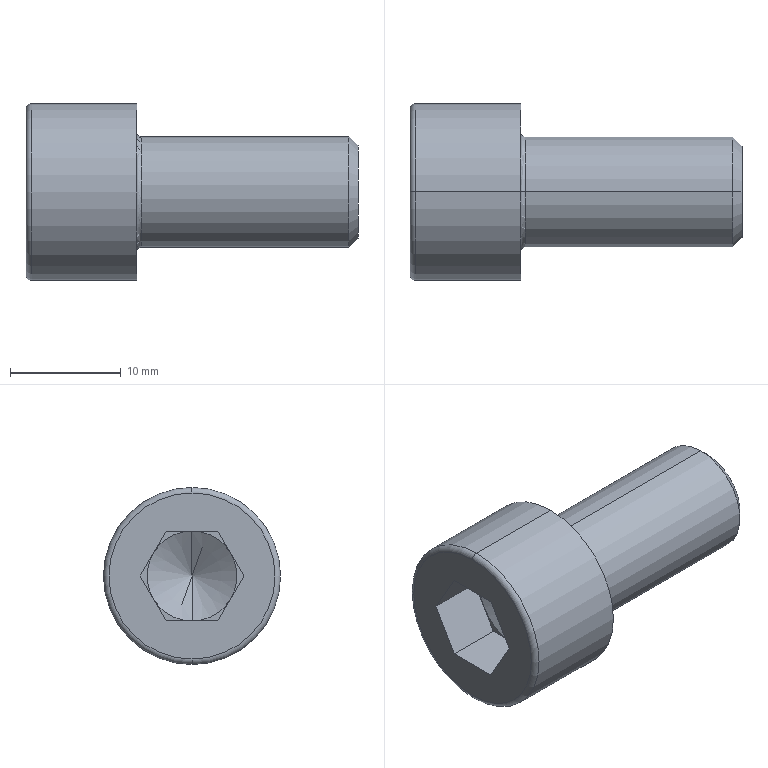Part | STEP file | PN_0067_socket head screw-M10x20L | 1 solid | 27 faces | box 30 x 16 x 16 mm | volume 3244 mm3 | plane 15 | cone 4 | torus 4 | cylinder 4 | commonest cylinder face diameters 10 x2 16 x2